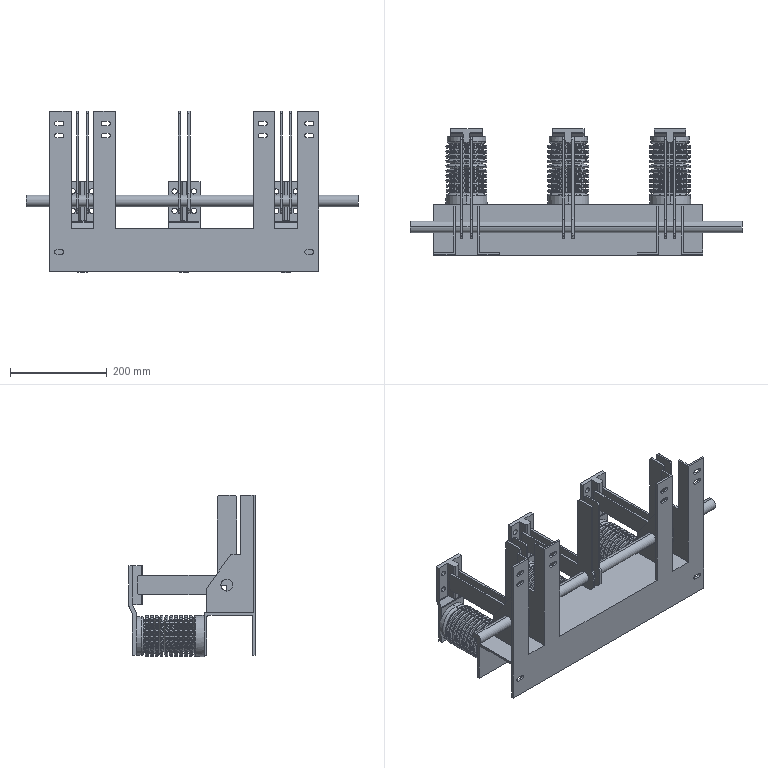Part | SolidWorks | features BaseBody 2 | 2 solids | 760 faces | box 685 x 260 x 332.5 mm | volume 4137959 mm3 | cylinder 320 | plane 242 | spline 132 | cone 66 | commonest cylinder face diameters 10 x85 65 x66 85 x66 11 x36 24 x27 9 x20